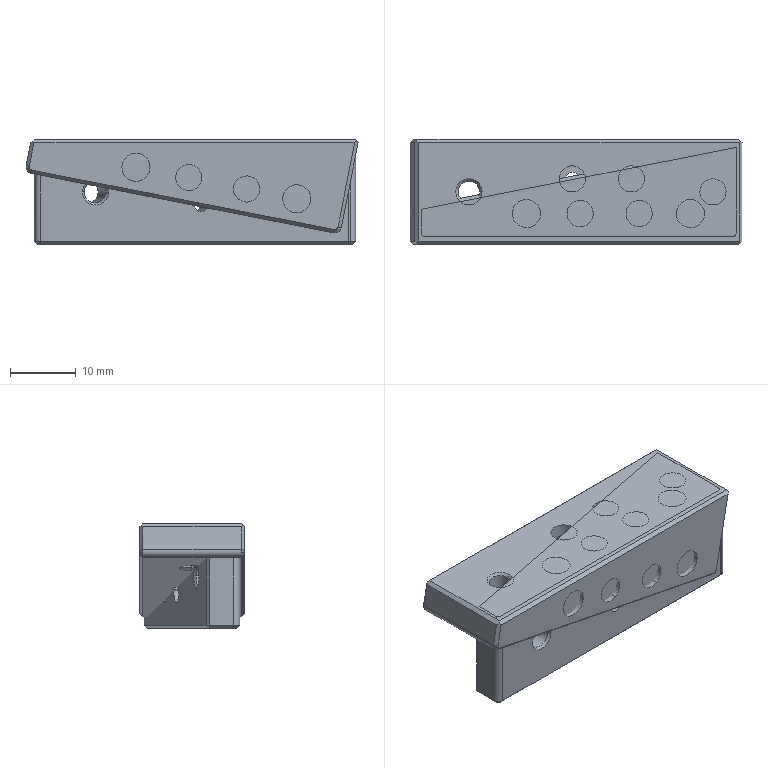NC program | NX | posted with a generic post | part box 50.629 x 16.001 x 16.002 mm
Whole program:
N10 G17 G21 G94 G90
(FLOOR_WALL_COPY , TOOL : D63)
N12 T01 M6
N14 G54
N16 G17 G0 G90 X7.302 Y34.5 S6500 M3
N18 G43 Z30. H1
N20 X7.3 Z6.201
N22 G94 G1 Z3.201 F1250.
N24 Y31.5
N26 Y-80.485 Z3.199
N28 Y-83.485
N30 Z6.199
N32 G0 X7.302 Z29.998
N34 Y34.5 Z30.
N36 X7.3 Z5.401
N38 G1 Z2.401
N40 Y31.5
N42 Y-80.485 Z2.399
N44 Y-83.485
N46 Z5.399
N48 G0 X7.302 Z29.998
N50 Y34.5 Z30.
N52 X7.3 Z4.601
N54 G1 Z1.601
N56 Y31.5
N58 Y-80.485 Z1.599
N60 Y-83.485
N62 Z4.599
N64 G0 X7.302 Z29.998
N66 Y34.5 Z30.
N68 X7.3 Z3.8
N70 G1 Z0.8
N72 Y31.5
N74 Y-80.485 Z0.798
N76 Y-83.485
N78 Z3.798
N80 G0 X7.302 Z29.998
N82 Y34.5 Z30.
N84 X7.3 Z3.
N86 G1 Z0.
N88 Y31.5
N90 Y-80.485 Z-0.002
N92 Y-83.485
N94 Z2.998
N96 G0 X7.302 Z29.998
N98 M5
(ZLEVEL_PROFILE_1_COPY_1_COPY_COPY_COPY , TOOL : D4A45)
N100 T02 M6
N102 G54
N104 G17 G0 G90 X3.632 Y-7.371 S9500 M3
N106 G43 Z30. H2
N108 Z-0.001
N110 G94 G1 Z-1.001 F1000.
N112 X3.011 Y-7.153
N114 G3 X2.811 Y-7.499 R0.4
N116 X4. Y-8.689 R1.189
N118 X2.811 Y-7.499 R-1.189
N120 X3.011 Y-7.846 R0.4
N122 G1 X3.632 Y-7.628
N124 Z-0.001
N126 G0 Z30.
N128 X3.633 Y-32.371 Z29.999
N130 Z-0.001
N132 G1 Z-1.001
N134 X3.011 Y-32.154
N136 G3 X2.811 Y-32.5 R0.4
N138 X4. Y-33.689 R1.189
N140 X2.811 Y-32.5 R-1.189
N142 X3.011 Y-32.846 R0.4
N144 G1 X3.633 Y-32.629
N146 Z-0.001
N148 G0 Z29.999
N150 X15.86 Y0.092
N152 Z-0.001
N154 G1 Z-1.001
N156 X15.348 Y-0.083
N158 G3 X15.085 Y-0.384 R0.4
N160 G1 X5.555 Y-48.866
N162 G2 X4.855 Y-49.442 R0.713
N164 G1 X1.005 Y-49.443
N166 G2 X-0.458 Y-47.98 R1.463
N168 G1 X-0.459 Y-1.002
N170 G2 X1.002 Y0.459 R1.461
N172 G1 X14.393 Y0.457
N174 G2 X15.085 Y-0.384 R0.705
N176 G3 X15.215 Y-0.762 R0.4
N178 G1 X15.737 Y-1.218
N180 Z-0.001
N182 G0 Z29.999
N184 M5
N186 M2